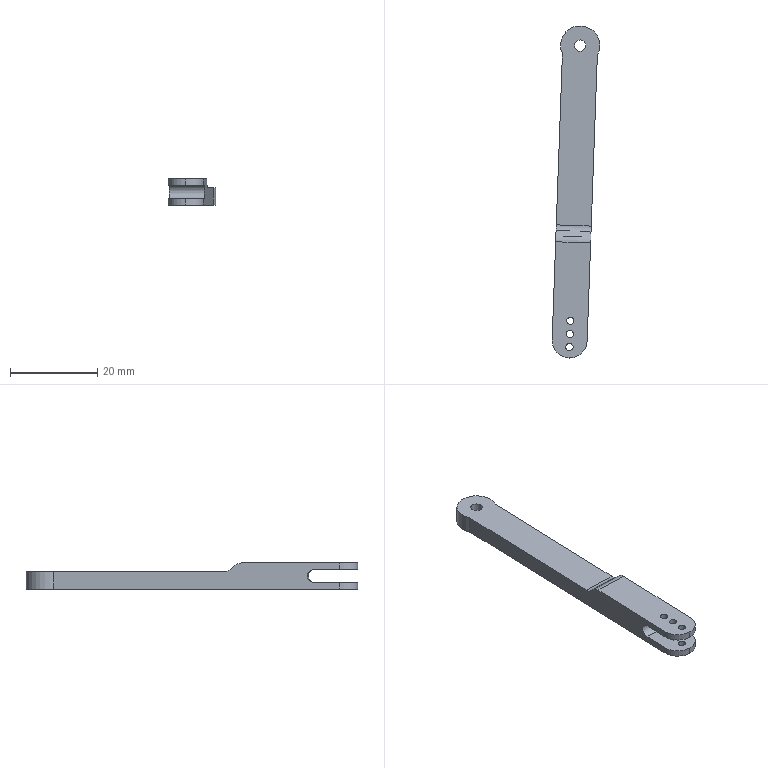Part | STEP file | Wytnij-wyci_gni_cie3 | 1 solid | 23 faces | box 10.909 x 75.957 x 6 mm | volume 2529 mm3 | cylinder 15 | plane 8 | commonest cylinder face diameters 1.67 x6 8 x4 4 x2 2.6 x1 3 x1 9 x1